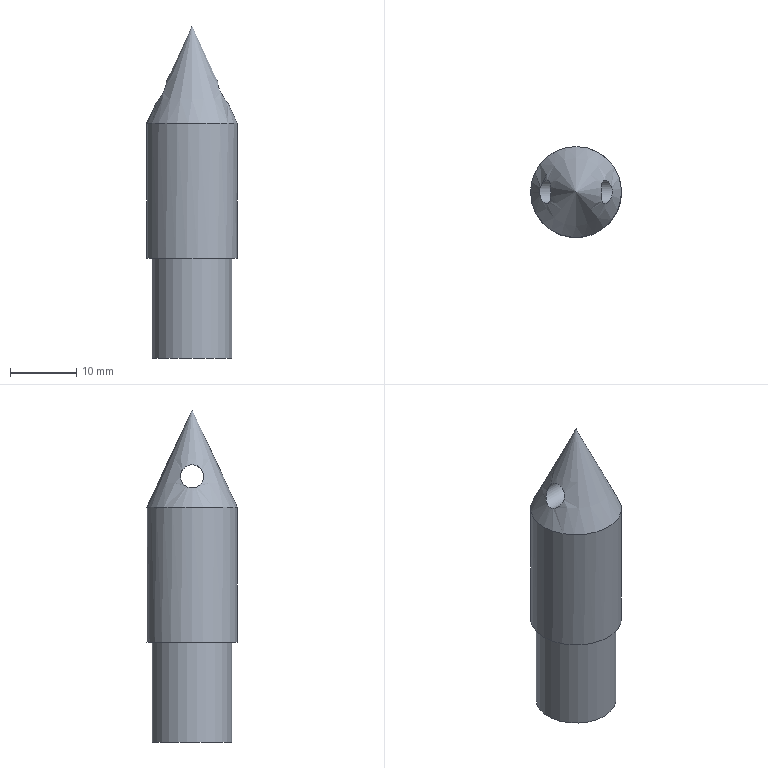Part | NX | features solid 2 | 1 solid | 6 faces | box 13.7 x 13.7 x 50 mm | volume 5325 mm3 | cylinder 3 | plane 2 | cone 1 | commonest cylinder face diameters 3.5 x1 12 x1 13.7 x1
STEP:
#1=CARTESIAN_POINT('',(-388.316,14.698,13.469));
#2=VERTEX_POINT('',#1);
#3=CARTESIAN_POINT('',(-388.563,13.206,13.149));
#4=CARTESIAN_POINT('',(-388.426,14.835,13.319));
#5=CARTESIAN_POINT('',(-387.629,15.645,14.385));
#6=CARTESIAN_POINT('',(-386.923,15.638,15.769));
#7=CARTESIAN_POINT('',(-386.845,14.476,16.871));
#8=CARTESIAN_POINT('',(-386.822,12.875,16.712));
#9=CARTESIAN_POINT('',(-387.045,11.965,15.424));
#10=CARTESIAN_POINT('',(-387.825,12.176,14.106));
#11=CARTESIAN_POINT('',(-388.563,13.206,13.149));
#12=CARTESIAN_POINT('',(-388.426,14.835,13.319));
#13=CARTESIAN_POINT('',(-387.629,15.645,14.385));
#14=B_SPLINE_CURVE_WITH_KNOTS('',3,(#3,#4,#5,#6,#7,#8,#9,#10,#11,#12,#13),.UNSPECIFIED.,.T.,.F.,(1,1,1,1,1,1,1,1,1,1,1,1,1,1,1),(-0.00435,-0.0029,-0.00145,0.,0.00145,0.0029,0.00435,0.0058,0.00725,0.0087,0.01015,0.0116,0.01305,0.0145,0.01595),.UNSPECIFIED.);
#15=EDGE_CURVE('',#2,#2,#14,.T.);
#16=ORIENTED_EDGE('',*,*,#15,.T.);
#17=EDGE_LOOP('',(#16));
#18=FACE_BOUND('',#17,.T.);
#19=CARTESIAN_POINT('',(-379.136,14.8,16.47));
#20=VERTEX_POINT('',#19);
#21=CARTESIAN_POINT('',(-379.152,13.335,16.906));
#22=CARTESIAN_POINT('',(-379.188,14.929,16.649));
#23=CARTESIAN_POINT('',(-378.914,15.752,15.32));
#24=CARTESIAN_POINT('',(-378.123,15.485,14.03));
#25=CARTESIAN_POINT('',(-377.413,14.392,13.115));
#26=CARTESIAN_POINT('',(-377.621,12.789,13.373));
#27=CARTESIAN_POINT('',(-378.43,12.03,14.466));
#28=CARTESIAN_POINT('',(-379.108,12.106,15.867));
#29=CARTESIAN_POINT('',(-379.152,13.335,16.906));
#30=CARTESIAN_POINT('',(-379.188,14.929,16.649));
#31=CARTESIAN_POINT('',(-378.914,15.752,15.32));
#32=B_SPLINE_CURVE_WITH_KNOTS('',3,(#21,#22,#23,#24,#25,#26,#27,#28,#29,#30,#31),.UNSPECIFIED.,.T.,.F.,(1,1,1,1,1,1,1,1,1,1,1,1,1,1,1),(-0.004355,-0.002903,-0.001452,0.,0.001452,0.002903,0.004355,0.005806,0.007258,0.008709,0.01016,0.01161,0.01306,0.01452,0.01597),.UNSPECIFIED.);
#33=EDGE_CURVE('',#20,#20,#32,.T.);
#34=ORIENTED_EDGE('',*,*,#33,.T.);
#35=EDGE_LOOP('',(#34));
#36=FACE_BOUND('',#35,.T.);
#37=CARTESIAN_POINT('',(-389.852,13.851,10.321));
#38=VERTEX_POINT('',#37);
#39=CARTESIAN_POINT('',(-383.002,13.851,10.321));
#40=DIRECTION('',(0.,0.,-1.));
#41=DIRECTION('',(-1.,0.,0.));
#42=AXIS2_PLACEMENT_3D('',#39,#40,#41);
#43=CIRCLE('',#42,6.85);
#44=EDGE_CURVE('',#38,#38,#43,.T.);
#45=ORIENTED_EDGE('',*,*,#44,.F.);
#46=EDGE_LOOP('',(#45));
#47=FACE_BOUND('',#46,.T.);
#48=CARTESIAN_POINT('',(-383.002,13.851,25.));
#49=VERTEX_POINT('',#48);
#50=VERTEX_LOOP('',#49);
#51=FACE_BOUND('',#50,.T.);
#52=CARTESIAN_POINT('',(-383.002,13.851,25.));
#53=DIRECTION('',(0.,0.,-1.));
#54=DIRECTION('',(0.,1.,0.));
#55=AXIS2_PLACEMENT_3D('',#52,#53,#54);
#56=CONICAL_SURFACE('',#55,0.,0.4366);
#57=ADVANCED_FACE('',(#18,#36,#47,#51),#56,.T.);
#58=CARTESIAN_POINT('',(-389.852,13.851,-10.));
#59=VERTEX_POINT('',#58);
#60=CARTESIAN_POINT('',(-383.002,13.851,-10.));
#61=DIRECTION('',(0.,0.,-1.));
#62=DIRECTION('',(-1.,0.,0.));
#63=AXIS2_PLACEMENT_3D('',#60,#61,#62);
#64=CIRCLE('',#63,6.85);
#65=EDGE_CURVE('',#59,#59,#64,.T.);
#66=ORIENTED_EDGE('',*,*,#65,.F.);
#67=EDGE_LOOP('',(#66));
#68=FACE_BOUND('',#67,.T.);
#69=ORIENTED_EDGE('',*,*,#44,.T.);
#70=EDGE_LOOP('',(#69));
#71=FACE_BOUND('',#70,.T.);
#72=CARTESIAN_POINT('',(-383.002,13.851,-25.));
#73=DIRECTION('',(0.,0.,-1.));
#74=DIRECTION('',(0.,1.,0.));
#75=AXIS2_PLACEMENT_3D('',#72,#73,#74);
#76=CYLINDRICAL_SURFACE('',#75,6.85);
#77=ADVANCED_FACE('',(#68,#71),#76,.T.);
#78=CARTESIAN_POINT('',(-383.002,19.851,-25.));
#79=VERTEX_POINT('',#78);
#80=CARTESIAN_POINT('',(-383.002,13.851,-25.));
#81=DIRECTION('',(0.,0.,-1.));
#82=DIRECTION('',(0.,1.,0.));
#83=AXIS2_PLACEMENT_3D('',#80,#81,#82);
#84=CIRCLE('',#83,6.);
#85=EDGE_CURVE('',#79,#79,#84,.T.);
#86=ORIENTED_EDGE('',*,*,#85,.F.);
#87=EDGE_LOOP('',(#86));
#88=FACE_BOUND('',#87,.T.);
#89=CARTESIAN_POINT('',(-383.002,19.851,-10.));
#90=VERTEX_POINT('',#89);
#91=CARTESIAN_POINT('',(-383.002,13.851,-10.));
#92=DIRECTION('',(0.,0.,-1.));
#93=DIRECTION('',(0.,1.,0.));
#94=AXIS2_PLACEMENT_3D('',#91,#92,#93);
#95=CIRCLE('',#94,6.);
#96=EDGE_CURVE('',#90,#90,#95,.T.);
#97=ORIENTED_EDGE('',*,*,#96,.T.);
#98=EDGE_LOOP('',(#97));
#99=FACE_BOUND('',#98,.T.);
#100=CARTESIAN_POINT('',(-383.002,13.851,-25.));
#101=DIRECTION('',(0.,0.,-1.));
#102=DIRECTION('',(0.,1.,0.));
#103=AXIS2_PLACEMENT_3D('',#100,#101,#102);
#104=CYLINDRICAL_SURFACE('',#103,6.);
#105=ADVANCED_FACE('',(#88,#99),#104,.T.);
#106=ORIENTED_EDGE('',*,*,#65,.T.);
#107=EDGE_LOOP('',(#106));
#108=FACE_BOUND('',#107,.T.);
#109=ORIENTED_EDGE('',*,*,#96,.F.);
#110=EDGE_LOOP('',(#109));
#111=FACE_BOUND('',#110,.T.);
#112=CARTESIAN_POINT('',(-377.002,13.851,-10.));
#113=DIRECTION('',(0.,0.,-1.));
#114=DIRECTION('',(0.,1.,0.));
#115=AXIS2_PLACEMENT_3D('',#112,#113,#114);
#116=PLANE('',#115);
#117=ADVANCED_FACE('',(#108,#111),#116,.T.);
#118=ORIENTED_EDGE('',*,*,#85,.T.);
#119=EDGE_LOOP('',(#118));
#120=FACE_BOUND('',#119,.T.);
#121=CARTESIAN_POINT('',(-383.002,13.851,-25.));
#122=DIRECTION('',(0.,0.,-1.));
#123=DIRECTION('',(0.,1.,0.));
#124=AXIS2_PLACEMENT_3D('',#121,#122,#123);
#125=PLANE('',#124);
#126=ADVANCED_FACE('',(#120),#125,.T.);
#127=ORIENTED_EDGE('',*,*,#33,.F.);
#128=EDGE_LOOP('',(#127));
#129=FACE_BOUND('',#128,.T.);
#130=ORIENTED_EDGE('',*,*,#15,.F.);
#131=EDGE_LOOP('',(#130));
#132=FACE_BOUND('',#131,.T.);
#133=CARTESIAN_POINT('',(-876.002,13.851,15.));
#134=DIRECTION('',(1.,0.,0.));
#135=DIRECTION('',(0.,1.,0.));
#136=AXIS2_PLACEMENT_3D('',#133,#134,#135);
#137=CYLINDRICAL_SURFACE('',#136,1.75);
#138=ADVANCED_FACE('',(#129,#132),#137,.F.);
#139=CLOSED_SHELL('',(#57,#77,#105,#117,#126,#138));
#140=MANIFOLD_SOLID_BREP('',#139);
#141=(LENGTH_UNIT()NAMED_UNIT(*)SI_UNIT(.MILLI.,.METRE.));
#142=UNCERTAINTY_MEASURE_WITH_UNIT(LENGTH_MEASURE(0.0508),#141,'','');
#143=(NAMED_UNIT(*)PLANE_ANGLE_UNIT()SI_UNIT($,.RADIAN.));
#144=(NAMED_UNIT(*)SI_UNIT($,.STERADIAN.)SOLID_ANGLE_UNIT());
#145=(GEOMETRIC_REPRESENTATION_CONTEXT(3)GLOBAL_UNCERTAINTY_ASSIGNED_CONTEXT((#142))GLOBAL_UNIT_ASSIGNED_CONTEXT((#141,#143,#144))REPRESENTATION_CONTEXT('',''));
#146=ADVANCED_BREP_SHAPE_REPRESENTATION('',(#140),#145);